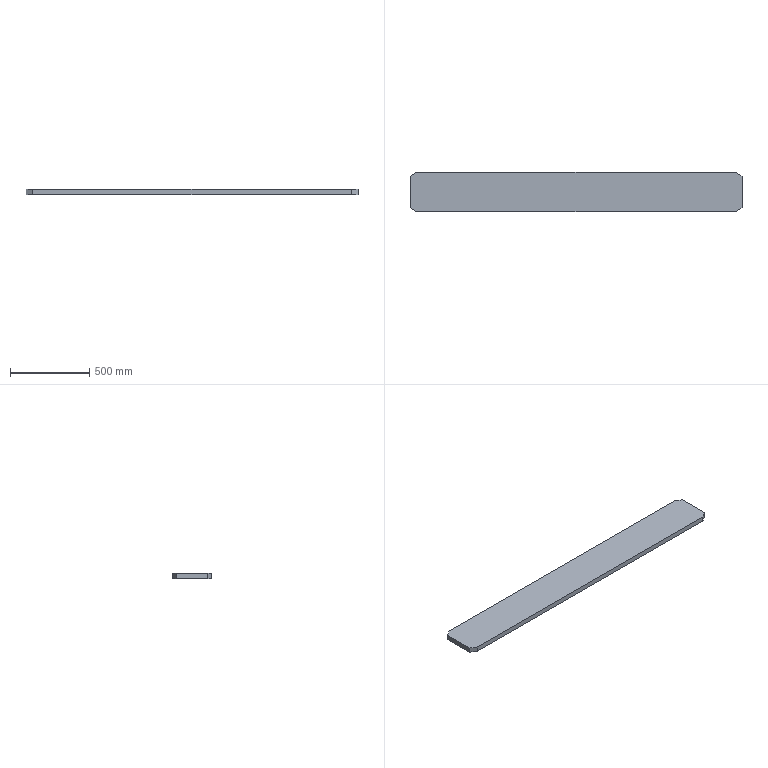Part | SolidWorks | features Extrusion 1 | 1 solid | 10 faces | box 2100 x 250 x 32 mm | volume 16730718 mm3 | plane 10
STEP:
#1=CARTESIAN_POINT('',(1006.699,-125.,-16.));
#2=VERTEX_POINT('',#1);
#3=CARTESIAN_POINT('',(1050.,-100.,-16.));
#4=VERTEX_POINT('',#3);
#5=CARTESIAN_POINT('',(1050.,-100.,-16.));
#6=DIRECTION('',(0.866,0.5,0.));
#7=VECTOR('',#6,1000.);
#8=LINE('',#5,#7);
#9=EDGE_CURVE('',#2,#4,#8,.T.);
#10=ORIENTED_EDGE('',*,*,#9,.T.);
#11=CARTESIAN_POINT('',(1050.,-100.,16.));
#12=VERTEX_POINT('',#11);
#13=CARTESIAN_POINT('',(1050.,-100.,16.));
#14=DIRECTION('',(0.,0.,-1.));
#15=VECTOR('',#14,1000.);
#16=LINE('',#13,#15);
#17=EDGE_CURVE('',#12,#4,#16,.T.);
#18=ORIENTED_EDGE('',*,*,#17,.F.);
#19=CARTESIAN_POINT('',(1006.699,-125.,16.));
#20=VERTEX_POINT('',#19);
#21=CARTESIAN_POINT('',(1050.,-100.,16.));
#22=DIRECTION('',(0.866,0.5,0.));
#23=VECTOR('',#22,1000.);
#24=LINE('',#21,#23);
#25=EDGE_CURVE('',#20,#12,#24,.T.);
#26=ORIENTED_EDGE('',*,*,#25,.F.);
#27=CARTESIAN_POINT('',(1006.699,-125.,16.));
#28=DIRECTION('',(0.,0.,-1.));
#29=VECTOR('',#28,1000.);
#30=LINE('',#27,#29);
#31=EDGE_CURVE('',#20,#2,#30,.T.);
#32=ORIENTED_EDGE('',*,*,#31,.T.);
#33=EDGE_LOOP('',(#10,#18,#26,#32));
#34=FACE_OUTER_BOUND('',#33,.T.);
#35=CARTESIAN_POINT('',(1050.,-100.,16.));
#36=DIRECTION('',(-0.5,0.866,0.));
#37=DIRECTION('',(-0.866,-0.5,0.));
#38=AXIS2_PLACEMENT_3D('',#35,#36,#37);
#39=PLANE('',#38);
#40=ADVANCED_FACE('',(#34),#39,.F.);
#41=CARTESIAN_POINT('',(1050.,100.,-16.));
#42=VERTEX_POINT('',#41);
#43=CARTESIAN_POINT('',(1050.,100.,-16.));
#44=DIRECTION('',(0.,1.,0.));
#45=VECTOR('',#44,1000.);
#46=LINE('',#43,#45);
#47=EDGE_CURVE('',#4,#42,#46,.T.);
#48=ORIENTED_EDGE('',*,*,#47,.T.);
#49=CARTESIAN_POINT('',(1050.,100.,16.));
#50=VERTEX_POINT('',#49);
#51=CARTESIAN_POINT('',(1050.,100.,16.));
#52=DIRECTION('',(0.,0.,-1.));
#53=VECTOR('',#52,1000.);
#54=LINE('',#51,#53);
#55=EDGE_CURVE('',#50,#42,#54,.T.);
#56=ORIENTED_EDGE('',*,*,#55,.F.);
#57=CARTESIAN_POINT('',(1050.,100.,16.));
#58=DIRECTION('',(0.,1.,0.));
#59=VECTOR('',#58,1000.);
#60=LINE('',#57,#59);
#61=EDGE_CURVE('',#12,#50,#60,.T.);
#62=ORIENTED_EDGE('',*,*,#61,.F.);
#63=ORIENTED_EDGE('',*,*,#17,.T.);
#64=EDGE_LOOP('',(#48,#56,#62,#63));
#65=FACE_OUTER_BOUND('',#64,.T.);
#66=CARTESIAN_POINT('',(1050.,100.,16.));
#67=DIRECTION('',(-1.,0.,0.));
#68=DIRECTION('',(0.,0.,1.));
#69=AXIS2_PLACEMENT_3D('',#66,#67,#68);
#70=PLANE('',#69);
#71=ADVANCED_FACE('',(#65),#70,.F.);
#72=CARTESIAN_POINT('',(1006.699,125.,-16.));
#73=VERTEX_POINT('',#72);
#74=CARTESIAN_POINT('',(1050.,100.,-16.));
#75=DIRECTION('',(-0.866,0.5,0.));
#76=VECTOR('',#75,1000.);
#77=LINE('',#74,#76);
#78=EDGE_CURVE('',#42,#73,#77,.T.);
#79=ORIENTED_EDGE('',*,*,#78,.T.);
#80=CARTESIAN_POINT('',(1006.699,125.,16.));
#81=VERTEX_POINT('',#80);
#82=CARTESIAN_POINT('',(1006.699,125.,16.));
#83=DIRECTION('',(0.,0.,-1.));
#84=VECTOR('',#83,1000.);
#85=LINE('',#82,#84);
#86=EDGE_CURVE('',#81,#73,#85,.T.);
#87=ORIENTED_EDGE('',*,*,#86,.F.);
#88=CARTESIAN_POINT('',(1050.,100.,16.));
#89=DIRECTION('',(-0.866,0.5,0.));
#90=VECTOR('',#89,1000.);
#91=LINE('',#88,#90);
#92=EDGE_CURVE('',#50,#81,#91,.T.);
#93=ORIENTED_EDGE('',*,*,#92,.F.);
#94=ORIENTED_EDGE('',*,*,#55,.T.);
#95=EDGE_LOOP('',(#79,#87,#93,#94));
#96=FACE_OUTER_BOUND('',#95,.T.);
#97=CARTESIAN_POINT('',(1050.,100.,16.));
#98=DIRECTION('',(-0.5,-0.866,0.));
#99=DIRECTION('',(0.866,-0.5,0.));
#100=AXIS2_PLACEMENT_3D('',#97,#98,#99);
#101=PLANE('',#100);
#102=ADVANCED_FACE('',(#96),#101,.F.);
#103=CARTESIAN_POINT('',(-1006.699,125.,-16.));
#104=VERTEX_POINT('',#103);
#105=CARTESIAN_POINT('',(-1006.699,125.,-16.));
#106=DIRECTION('',(-1.,0.,0.));
#107=VECTOR('',#106,1000.);
#108=LINE('',#105,#107);
#109=EDGE_CURVE('',#73,#104,#108,.T.);
#110=ORIENTED_EDGE('',*,*,#109,.T.);
#111=CARTESIAN_POINT('',(-1006.699,125.,16.));
#112=VERTEX_POINT('',#111);
#113=CARTESIAN_POINT('',(-1006.699,125.,16.));
#114=DIRECTION('',(0.,0.,-1.));
#115=VECTOR('',#114,1000.);
#116=LINE('',#113,#115);
#117=EDGE_CURVE('',#112,#104,#116,.T.);
#118=ORIENTED_EDGE('',*,*,#117,.F.);
#119=CARTESIAN_POINT('',(-1006.699,125.,16.));
#120=DIRECTION('',(-1.,0.,0.));
#121=VECTOR('',#120,1000.);
#122=LINE('',#119,#121);
#123=EDGE_CURVE('',#81,#112,#122,.T.);
#124=ORIENTED_EDGE('',*,*,#123,.F.);
#125=ORIENTED_EDGE('',*,*,#86,.T.);
#126=EDGE_LOOP('',(#110,#118,#124,#125));
#127=FACE_OUTER_BOUND('',#126,.T.);
#128=CARTESIAN_POINT('',(-1006.699,125.,16.));
#129=DIRECTION('',(0.,-1.,0.));
#130=DIRECTION('',(0.,0.,-1.));
#131=AXIS2_PLACEMENT_3D('',#128,#129,#130);
#132=PLANE('',#131);
#133=ADVANCED_FACE('',(#127),#132,.F.);
#134=CARTESIAN_POINT('',(-1050.,100.,-16.));
#135=VERTEX_POINT('',#134);
#136=CARTESIAN_POINT('',(-1050.,100.,-16.));
#137=DIRECTION('',(-0.866,-0.5,0.));
#138=VECTOR('',#137,1000.);
#139=LINE('',#136,#138);
#140=EDGE_CURVE('',#104,#135,#139,.T.);
#141=ORIENTED_EDGE('',*,*,#140,.T.);
#142=CARTESIAN_POINT('',(-1050.,100.,16.));
#143=VERTEX_POINT('',#142);
#144=CARTESIAN_POINT('',(-1050.,100.,16.));
#145=DIRECTION('',(0.,0.,-1.));
#146=VECTOR('',#145,1000.);
#147=LINE('',#144,#146);
#148=EDGE_CURVE('',#143,#135,#147,.T.);
#149=ORIENTED_EDGE('',*,*,#148,.F.);
#150=CARTESIAN_POINT('',(-1050.,100.,16.));
#151=DIRECTION('',(-0.866,-0.5,0.));
#152=VECTOR('',#151,1000.);
#153=LINE('',#150,#152);
#154=EDGE_CURVE('',#112,#143,#153,.T.);
#155=ORIENTED_EDGE('',*,*,#154,.F.);
#156=ORIENTED_EDGE('',*,*,#117,.T.);
#157=EDGE_LOOP('',(#141,#149,#155,#156));
#158=FACE_OUTER_BOUND('',#157,.T.);
#159=CARTESIAN_POINT('',(-1050.,100.,16.));
#160=DIRECTION('',(0.5,-0.866,0.));
#161=DIRECTION('',(0.866,0.5,0.));
#162=AXIS2_PLACEMENT_3D('',#159,#160,#161);
#163=PLANE('',#162);
#164=ADVANCED_FACE('',(#158),#163,.F.);
#165=CARTESIAN_POINT('',(-1050.,-100.,-16.));
#166=VERTEX_POINT('',#165);
#167=CARTESIAN_POINT('',(-1050.,100.,-16.));
#168=DIRECTION('',(0.,-1.,0.));
#169=VECTOR('',#168,1000.);
#170=LINE('',#167,#169);
#171=EDGE_CURVE('',#135,#166,#170,.T.);
#172=ORIENTED_EDGE('',*,*,#171,.T.);
#173=CARTESIAN_POINT('',(-1050.,-100.,16.));
#174=VERTEX_POINT('',#173);
#175=CARTESIAN_POINT('',(-1050.,-100.,16.));
#176=DIRECTION('',(0.,0.,-1.));
#177=VECTOR('',#176,1000.);
#178=LINE('',#175,#177);
#179=EDGE_CURVE('',#174,#166,#178,.T.);
#180=ORIENTED_EDGE('',*,*,#179,.F.);
#181=CARTESIAN_POINT('',(-1050.,100.,16.));
#182=DIRECTION('',(0.,-1.,0.));
#183=VECTOR('',#182,1000.);
#184=LINE('',#181,#183);
#185=EDGE_CURVE('',#143,#174,#184,.T.);
#186=ORIENTED_EDGE('',*,*,#185,.F.);
#187=ORIENTED_EDGE('',*,*,#148,.T.);
#188=EDGE_LOOP('',(#172,#180,#186,#187));
#189=FACE_OUTER_BOUND('',#188,.T.);
#190=CARTESIAN_POINT('',(-1050.,100.,16.));
#191=DIRECTION('',(1.,0.,0.));
#192=DIRECTION('',(0.,0.,-1.));
#193=AXIS2_PLACEMENT_3D('',#190,#191,#192);
#194=PLANE('',#193);
#195=ADVANCED_FACE('',(#189),#194,.F.);
#196=CARTESIAN_POINT('',(-1006.699,-125.,-16.));
#197=VERTEX_POINT('',#196);
#198=CARTESIAN_POINT('',(-1050.,-100.,-16.));
#199=DIRECTION('',(0.866,-0.5,0.));
#200=VECTOR('',#199,1000.);
#201=LINE('',#198,#200);
#202=EDGE_CURVE('',#166,#197,#201,.T.);
#203=ORIENTED_EDGE('',*,*,#202,.T.);
#204=CARTESIAN_POINT('',(-1006.699,-125.,16.));
#205=VERTEX_POINT('',#204);
#206=CARTESIAN_POINT('',(-1006.699,-125.,16.));
#207=DIRECTION('',(0.,0.,-1.));
#208=VECTOR('',#207,1000.);
#209=LINE('',#206,#208);
#210=EDGE_CURVE('',#205,#197,#209,.T.);
#211=ORIENTED_EDGE('',*,*,#210,.F.);
#212=CARTESIAN_POINT('',(-1050.,-100.,16.));
#213=DIRECTION('',(0.866,-0.5,0.));
#214=VECTOR('',#213,1000.);
#215=LINE('',#212,#214);
#216=EDGE_CURVE('',#174,#205,#215,.T.);
#217=ORIENTED_EDGE('',*,*,#216,.F.);
#218=ORIENTED_EDGE('',*,*,#179,.T.);
#219=EDGE_LOOP('',(#203,#211,#217,#218));
#220=FACE_OUTER_BOUND('',#219,.T.);
#221=CARTESIAN_POINT('',(-1050.,-100.,16.));
#222=DIRECTION('',(0.5,0.866,0.));
#223=DIRECTION('',(-0.866,0.5,0.));
#224=AXIS2_PLACEMENT_3D('',#221,#222,#223);
#225=PLANE('',#224);
#226=ADVANCED_FACE('',(#220),#225,.F.);
#227=CARTESIAN_POINT('',(-1006.699,-125.,-16.));
#228=DIRECTION('',(1.,0.,0.));
#229=VECTOR('',#228,1000.);
#230=LINE('',#227,#229);
#231=EDGE_CURVE('',#197,#2,#230,.T.);
#232=ORIENTED_EDGE('',*,*,#231,.T.);
#233=ORIENTED_EDGE('',*,*,#31,.F.);
#234=CARTESIAN_POINT('',(-1006.699,-125.,16.));
#235=DIRECTION('',(1.,0.,0.));
#236=VECTOR('',#235,1000.);
#237=LINE('',#234,#236);
#238=EDGE_CURVE('',#205,#20,#237,.T.);
#239=ORIENTED_EDGE('',*,*,#238,.F.);
#240=ORIENTED_EDGE('',*,*,#210,.T.);
#241=EDGE_LOOP('',(#232,#233,#239,#240));
#242=FACE_OUTER_BOUND('',#241,.T.);
#243=CARTESIAN_POINT('',(-1006.699,-125.,16.));
#244=DIRECTION('',(0.,1.,0.));
#245=DIRECTION('',(0.,0.,1.));
#246=AXIS2_PLACEMENT_3D('',#243,#244,#245);
#247=PLANE('',#246);
#248=ADVANCED_FACE('',(#242),#247,.F.);
#249=ORIENTED_EDGE('',*,*,#25,.T.);
#250=ORIENTED_EDGE('',*,*,#61,.T.);
#251=ORIENTED_EDGE('',*,*,#92,.T.);
#252=ORIENTED_EDGE('',*,*,#123,.T.);
#253=ORIENTED_EDGE('',*,*,#154,.T.);
#254=ORIENTED_EDGE('',*,*,#185,.T.);
#255=ORIENTED_EDGE('',*,*,#216,.T.);
#256=ORIENTED_EDGE('',*,*,#238,.T.);
#257=EDGE_LOOP('',(#249,#250,#251,#252,#253,#254,#255,#256));
#258=FACE_OUTER_BOUND('',#257,.T.);
#259=CARTESIAN_POINT('',(0.,-706.218,16.));
#260=DIRECTION('',(0.,0.,1.));
#261=DIRECTION('',(1.,0.,0.));
#262=AXIS2_PLACEMENT_3D('',#259,#260,#261);
#263=PLANE('',#262);
#264=ADVANCED_FACE('',(#258),#263,.T.);
#265=ORIENTED_EDGE('',*,*,#9,.F.);
#266=ORIENTED_EDGE('',*,*,#231,.F.);
#267=ORIENTED_EDGE('',*,*,#202,.F.);
#268=ORIENTED_EDGE('',*,*,#171,.F.);
#269=ORIENTED_EDGE('',*,*,#140,.F.);
#270=ORIENTED_EDGE('',*,*,#109,.F.);
#271=ORIENTED_EDGE('',*,*,#78,.F.);
#272=ORIENTED_EDGE('',*,*,#47,.F.);
#273=EDGE_LOOP('',(#265,#266,#267,#268,#269,#270,#271,#272));
#274=FACE_OUTER_BOUND('',#273,.T.);
#275=CARTESIAN_POINT('',(0.,-706.218,-16.));
#276=DIRECTION('',(0.,0.,1.));
#277=DIRECTION('',(1.,0.,0.));
#278=AXIS2_PLACEMENT_3D('',#275,#276,#277);
#279=PLANE('',#278);
#280=ADVANCED_FACE('',(#274),#279,.F.);
#281=CLOSED_SHELL('',(#40,#71,#102,#133,#164,#195,#226,#248,#264,#280));
#282=MANIFOLD_SOLID_BREP('',#281);
#283=CARTESIAN_POINT('',(0.,0.,0.));
#284=DIRECTION('',(0.,0.,1.));
#285=DIRECTION('',(1.,0.,0.));
#286=AXIS2_PLACEMENT_3D('',#283,#284,#285);
#287=(LENGTH_UNIT()NAMED_UNIT(*)SI_UNIT(.MILLI.,.METRE.));
#288=UNCERTAINTY_MEASURE_WITH_UNIT(LENGTH_MEASURE(0.00001),#287,'','');
#289=(NAMED_UNIT(*)PLANE_ANGLE_UNIT()SI_UNIT($,.RADIAN.));
#290=(NAMED_UNIT(*)SI_UNIT($,.STERADIAN.)SOLID_ANGLE_UNIT());
#291=(GEOMETRIC_REPRESENTATION_CONTEXT(3)GLOBAL_UNCERTAINTY_ASSIGNED_CONTEXT((#288))GLOBAL_UNIT_ASSIGNED_CONTEXT((#287,#289,#290))REPRESENTATION_CONTEXT('',''));
#292=ADVANCED_BREP_SHAPE_REPRESENTATION('',(#282,#286),#291);